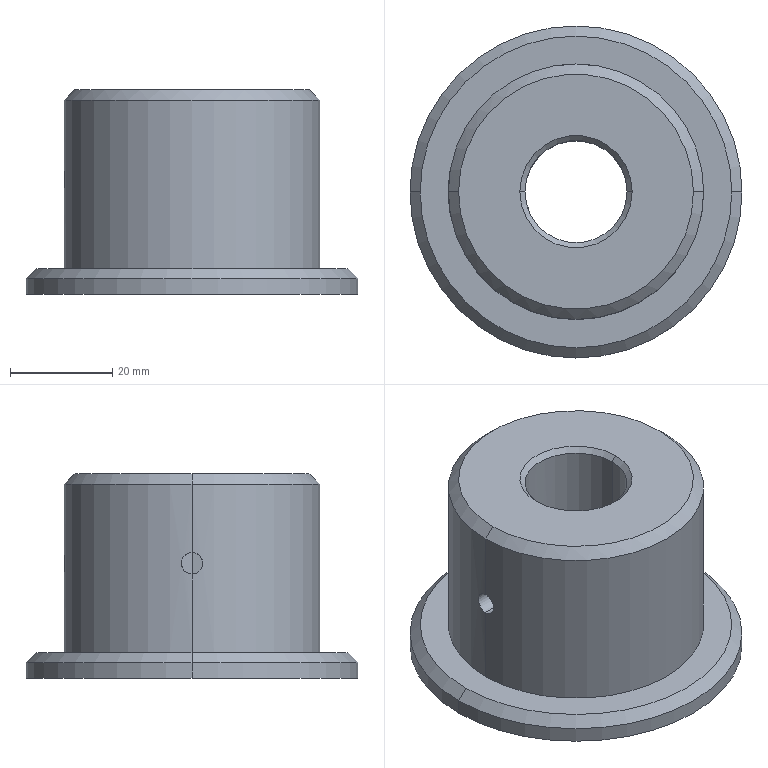Part | SolidWorks | features BaseBody 1 | 1 solid | 21 faces | box 65 x 65 x 40 mm | volume 71560 mm3 | cylinder 10 | cone 8 | plane 3 | commonest cylinder face diameters 4.2 x4 20 x2 50 x2 65 x2
STEP:
#1=CARTESIAN_POINT('',(0.,10.,24.6));
#2=VERTEX_POINT('',#1);
#3=CARTESIAN_POINT('',(0.,10.,20.4));
#4=VERTEX_POINT('',#3);
#5=CARTESIAN_POINT('',(0.,10.,24.6));
#6=CARTESIAN_POINT('',(-0.1391,10.,24.6));
#7=CARTESIAN_POINT('',(-0.2759,9.997,24.586));
#8=CARTESIAN_POINT('',(-0.5447,9.986,24.533));
#9=CARTESIAN_POINT('',(-0.6783,9.978,24.492));
#10=CARTESIAN_POINT('',(-0.9324,9.957,24.387));
#11=CARTESIAN_POINT('',(-1.053,9.945,24.322));
#12=CARTESIAN_POINT('',(-1.281,9.918,24.17));
#13=CARTESIAN_POINT('',(-1.388,9.904,24.081));
#14=CARTESIAN_POINT('',(-1.678,9.86,23.792));
#15=CARTESIAN_POINT('',(-1.834,9.831,23.558));
#16=CARTESIAN_POINT('',(-1.992,9.8,23.179));
#17=CARTESIAN_POINT('',(-2.032,9.791,23.047));
#18=CARTESIAN_POINT('',(-2.086,9.78,22.776));
#19=CARTESIAN_POINT('',(-2.1,9.777,22.639));
#20=CARTESIAN_POINT('',(-2.1,9.777,22.364));
#21=CARTESIAN_POINT('',(-2.086,9.78,22.225));
#22=CARTESIAN_POINT('',(-2.033,9.791,21.955));
#23=CARTESIAN_POINT('',(-1.993,9.8,21.824));
#24=CARTESIAN_POINT('',(-1.835,9.831,21.442));
#25=CARTESIAN_POINT('',(-1.681,9.86,21.211));
#26=CARTESIAN_POINT('',(-1.388,9.904,20.918));
#27=CARTESIAN_POINT('',(-1.283,9.918,20.832));
#28=CARTESIAN_POINT('',(-1.056,9.945,20.68));
#29=CARTESIAN_POINT('',(-0.9328,9.957,20.614));
#30=CARTESIAN_POINT('',(-0.6792,9.978,20.508));
#31=CARTESIAN_POINT('',(-0.5483,9.986,20.468));
#32=CARTESIAN_POINT('',(-0.2784,9.997,20.414));
#33=CARTESIAN_POINT('',(-0.1391,10.,20.4));
#34=CARTESIAN_POINT('',(0.,10.,20.4));
#35=B_SPLINE_CURVE_WITH_KNOTS('',3,(#5,#6,#7,#8,#9,#10,#11,#12,#13,#14,#15,#16,#17,#18,#19,#20,#21,#22,#23,#24,#25,#26,#27,#28,#29,#30,#31,#32,#33,#34),.UNSPECIFIED.,.F.,.F.,(4,2,2,2,2,2,2,2,2,2,2,2,2,2,4),(0.,0.0004114,0.0008228,0.001234,0.001646,0.002468,0.00288,0.003291,0.003702,0.004114,0.004937,0.005348,0.005759,0.006171,0.006582),.UNSPECIFIED.);
#36=EDGE_CURVE('',#2,#4,#35,.T.);
#37=ORIENTED_EDGE('',*,*,#36,.T.);
#38=CARTESIAN_POINT('',(0.,25.,20.4));
#39=VERTEX_POINT('',#38);
#40=CARTESIAN_POINT('',(0.,25.,20.4));
#41=DIRECTION('',(0.,1.,0.));
#42=VECTOR('',#41,1000.);
#43=LINE('',#40,#42);
#44=EDGE_CURVE('',#4,#39,#43,.T.);
#45=ORIENTED_EDGE('',*,*,#44,.T.);
#46=CARTESIAN_POINT('',(0.,25.,24.6));
#47=VERTEX_POINT('',#46);
#48=CARTESIAN_POINT('',(0.,25.,24.6));
#49=CARTESIAN_POINT('',(-0.1388,25.,24.6));
#50=CARTESIAN_POINT('',(-0.2752,24.999,24.586));
#51=CARTESIAN_POINT('',(-0.5437,24.994,24.533));
#52=CARTESIAN_POINT('',(-0.6771,24.991,24.493));
#53=CARTESIAN_POINT('',(-0.9313,24.983,24.387));
#54=CARTESIAN_POINT('',(-1.052,24.978,24.323));
#55=CARTESIAN_POINT('',(-1.28,24.967,24.17));
#56=CARTESIAN_POINT('',(-1.388,24.962,24.082));
#57=CARTESIAN_POINT('',(-1.679,24.944,23.791));
#58=CARTESIAN_POINT('',(-1.835,24.933,23.557));
#59=CARTESIAN_POINT('',(-2.045,24.916,23.052));
#60=CARTESIAN_POINT('',(-2.1,24.912,22.775));
#61=CARTESIAN_POINT('',(-2.1,24.912,22.364));
#62=CARTESIAN_POINT('',(-2.086,24.913,22.225));
#63=CARTESIAN_POINT('',(-2.033,24.917,21.956));
#64=CARTESIAN_POINT('',(-1.993,24.92,21.825));
#65=CARTESIAN_POINT('',(-1.888,24.929,21.571));
#66=CARTESIAN_POINT('',(-1.823,24.934,21.448));
#67=CARTESIAN_POINT('',(-1.671,24.944,21.22));
#68=CARTESIAN_POINT('',(-1.584,24.95,21.114));
#69=CARTESIAN_POINT('',(-1.388,24.962,20.918));
#70=CARTESIAN_POINT('',(-1.282,24.967,20.831));
#71=CARTESIAN_POINT('',(-1.055,24.978,20.679));
#72=CARTESIAN_POINT('',(-0.932,24.983,20.613));
#73=CARTESIAN_POINT('',(-0.6777,24.991,20.508));
#74=CARTESIAN_POINT('',(-0.5468,24.994,20.468));
#75=CARTESIAN_POINT('',(-0.2777,24.999,20.414));
#76=CARTESIAN_POINT('',(-0.1388,25.,20.4));
#77=CARTESIAN_POINT('',(0.,25.,20.4));
#78=B_SPLINE_CURVE_WITH_KNOTS('',3,(#48,#49,#50,#51,#52,#53,#54,#55,#56,#57,#58,#59,#60,#61,#62,#63,#64,#65,#66,#67,#68,#69,#70,#71,#72,#73,#74,#75,#76,#77),.UNSPECIFIED.,.F.,.F.,(4,2,2,2,2,2,2,2,2,2,2,2,2,2,4),(0.,0.0004104,0.0008209,0.001231,0.001642,0.002463,0.003284,0.003694,0.004104,0.004515,0.004925,0.005336,0.005746,0.006157,0.006567),.UNSPECIFIED.);
#79=EDGE_CURVE('',#47,#39,#78,.T.);
#80=ORIENTED_EDGE('',*,*,#79,.F.);
#81=CARTESIAN_POINT('',(0.,25.,24.6));
#82=DIRECTION('',(0.,1.,0.));
#83=VECTOR('',#82,1000.);
#84=LINE('',#81,#83);
#85=EDGE_CURVE('',#2,#47,#84,.T.);
#86=ORIENTED_EDGE('',*,*,#85,.F.);
#87=EDGE_LOOP('',(#37,#45,#80,#86));
#88=FACE_OUTER_BOUND('',#87,.T.);
#89=CARTESIAN_POINT('',(0.,25.,22.5));
#90=DIRECTION('',(0.,1.,0.));
#91=DIRECTION('',(0.,0.,1.));
#92=AXIS2_PLACEMENT_3D('',#89,#90,#91);
#93=CYLINDRICAL_SURFACE('',#92,2.1);
#94=ADVANCED_FACE('',(#88),#93,.F.);
#95=CARTESIAN_POINT('',(-10.,0.,24.6));
#96=VERTEX_POINT('',#95);
#97=CARTESIAN_POINT('',(-10.,0.,20.4));
#98=VERTEX_POINT('',#97);
#99=CARTESIAN_POINT('',(-10.,0.,24.6));
#100=CARTESIAN_POINT('',(-10.,-0.1391,24.6));
#101=CARTESIAN_POINT('',(-9.997,-0.2759,24.586));
#102=CARTESIAN_POINT('',(-9.986,-0.5447,24.533));
#103=CARTESIAN_POINT('',(-9.978,-0.6783,24.492));
#104=CARTESIAN_POINT('',(-9.957,-0.9324,24.387));
#105=CARTESIAN_POINT('',(-9.945,-1.053,24.322));
#106=CARTESIAN_POINT('',(-9.918,-1.281,24.17));
#107=CARTESIAN_POINT('',(-9.904,-1.388,24.081));
#108=CARTESIAN_POINT('',(-9.86,-1.678,23.792));
#109=CARTESIAN_POINT('',(-9.831,-1.834,23.558));
#110=CARTESIAN_POINT('',(-9.8,-1.992,23.179));
#111=CARTESIAN_POINT('',(-9.791,-2.032,23.047));
#112=CARTESIAN_POINT('',(-9.78,-2.086,22.776));
#113=CARTESIAN_POINT('',(-9.777,-2.1,22.639));
#114=CARTESIAN_POINT('',(-9.777,-2.1,22.364));
#115=CARTESIAN_POINT('',(-9.78,-2.086,22.225));
#116=CARTESIAN_POINT('',(-9.791,-2.033,21.955));
#117=CARTESIAN_POINT('',(-9.8,-1.993,21.824));
#118=CARTESIAN_POINT('',(-9.831,-1.835,21.442));
#119=CARTESIAN_POINT('',(-9.86,-1.681,21.211));
#120=CARTESIAN_POINT('',(-9.904,-1.388,20.918));
#121=CARTESIAN_POINT('',(-9.918,-1.283,20.832));
#122=CARTESIAN_POINT('',(-9.945,-1.056,20.68));
#123=CARTESIAN_POINT('',(-9.957,-0.9328,20.614));
#124=CARTESIAN_POINT('',(-9.978,-0.6792,20.508));
#125=CARTESIAN_POINT('',(-9.986,-0.5483,20.468));
#126=CARTESIAN_POINT('',(-9.997,-0.2784,20.414));
#127=CARTESIAN_POINT('',(-10.,-0.1391,20.4));
#128=CARTESIAN_POINT('',(-10.,0.,20.4));
#129=B_SPLINE_CURVE_WITH_KNOTS('',3,(#99,#100,#101,#102,#103,#104,#105,#106,#107,#108,#109,#110,#111,#112,#113,#114,#115,#116,#117,#118,#119,#120,#121,#122,#123,#124,#125,#126,#127,#128),.UNSPECIFIED.,.F.,.F.,(4,2,2,2,2,2,2,2,2,2,2,2,2,2,4),(0.,0.0004114,0.0008228,0.001234,0.001646,0.002468,0.00288,0.003291,0.003702,0.004114,0.004937,0.005348,0.005759,0.006171,0.006582),.UNSPECIFIED.);
#130=EDGE_CURVE('',#96,#98,#129,.T.);
#131=ORIENTED_EDGE('',*,*,#130,.T.);
#132=CARTESIAN_POINT('',(-25.,0.,20.4));
#133=VERTEX_POINT('',#132);
#134=CARTESIAN_POINT('',(-25.,0.,20.4));
#135=DIRECTION('',(-1.,0.,0.));
#136=VECTOR('',#135,1000.);
#137=LINE('',#134,#136);
#138=EDGE_CURVE('',#98,#133,#137,.T.);
#139=ORIENTED_EDGE('',*,*,#138,.T.);
#140=CARTESIAN_POINT('',(-25.,0.,24.6));
#141=VERTEX_POINT('',#140);
#142=CARTESIAN_POINT('',(-25.,0.,24.6));
#143=CARTESIAN_POINT('',(-25.,-0.1388,24.6));
#144=CARTESIAN_POINT('',(-24.999,-0.2752,24.586));
#145=CARTESIAN_POINT('',(-24.994,-0.5437,24.533));
#146=CARTESIAN_POINT('',(-24.991,-0.6771,24.493));
#147=CARTESIAN_POINT('',(-24.983,-0.9313,24.387));
#148=CARTESIAN_POINT('',(-24.978,-1.052,24.323));
#149=CARTESIAN_POINT('',(-24.967,-1.28,24.17));
#150=CARTESIAN_POINT('',(-24.962,-1.388,24.082));
#151=CARTESIAN_POINT('',(-24.944,-1.679,23.791));
#152=CARTESIAN_POINT('',(-24.933,-1.835,23.557));
#153=CARTESIAN_POINT('',(-24.916,-2.045,23.052));
#154=CARTESIAN_POINT('',(-24.912,-2.1,22.775));
#155=CARTESIAN_POINT('',(-24.912,-2.1,22.364));
#156=CARTESIAN_POINT('',(-24.913,-2.086,22.225));
#157=CARTESIAN_POINT('',(-24.917,-2.033,21.956));
#158=CARTESIAN_POINT('',(-24.92,-1.993,21.825));
#159=CARTESIAN_POINT('',(-24.929,-1.888,21.571));
#160=CARTESIAN_POINT('',(-24.934,-1.823,21.448));
#161=CARTESIAN_POINT('',(-24.944,-1.671,21.22));
#162=CARTESIAN_POINT('',(-24.95,-1.584,21.114));
#163=CARTESIAN_POINT('',(-24.962,-1.388,20.918));
#164=CARTESIAN_POINT('',(-24.967,-1.282,20.831));
#165=CARTESIAN_POINT('',(-24.978,-1.055,20.679));
#166=CARTESIAN_POINT('',(-24.983,-0.932,20.613));
#167=CARTESIAN_POINT('',(-24.991,-0.6777,20.508));
#168=CARTESIAN_POINT('',(-24.994,-0.5468,20.468));
#169=CARTESIAN_POINT('',(-24.999,-0.2777,20.414));
#170=CARTESIAN_POINT('',(-25.,-0.1388,20.4));
#171=CARTESIAN_POINT('',(-25.,0.,20.4));
#172=B_SPLINE_CURVE_WITH_KNOTS('',3,(#142,#143,#144,#145,#146,#147,#148,#149,#150,#151,#152,#153,#154,#155,#156,#157,#158,#159,#160,#161,#162,#163,#164,#165,#166,#167,#168,#169,#170,#171),.UNSPECIFIED.,.F.,.F.,(4,2,2,2,2,2,2,2,2,2,2,2,2,2,4),(0.,0.0004104,0.0008209,0.001231,0.001642,0.002463,0.003284,0.003694,0.004104,0.004515,0.004925,0.005336,0.005746,0.006157,0.006567),.UNSPECIFIED.);
#173=EDGE_CURVE('',#141,#133,#172,.T.);
#174=ORIENTED_EDGE('',*,*,#173,.F.);
#175=CARTESIAN_POINT('',(-25.,0.,24.6));
#176=DIRECTION('',(-1.,0.,0.));
#177=VECTOR('',#176,1000.);
#178=LINE('',#175,#177);
#179=EDGE_CURVE('',#96,#141,#178,.T.);
#180=ORIENTED_EDGE('',*,*,#179,.F.);
#181=EDGE_LOOP('',(#131,#139,#174,#180));
#182=FACE_OUTER_BOUND('',#181,.T.);
#183=CARTESIAN_POINT('',(-25.,0.,22.5));
#184=DIRECTION('',(-1.,0.,0.));
#185=DIRECTION('',(0.,0.,1.));
#186=AXIS2_PLACEMENT_3D('',#183,#184,#185);
#187=CYLINDRICAL_SURFACE('',#186,2.1);
#188=ADVANCED_FACE('',(#182),#187,.F.);
#189=CARTESIAN_POINT('',(10.,0.,1.));
#190=VERTEX_POINT('',#189);
#191=CARTESIAN_POINT('',(-10.,0.,1.));
#192=VERTEX_POINT('',#191);
#193=CARTESIAN_POINT('',(0.,0.,1.));
#194=DIRECTION('',(0.,0.,-1.));
#195=DIRECTION('',(1.,0.,0.));
#196=AXIS2_PLACEMENT_3D('',#193,#194,#195);
#197=CIRCLE('',#196,10.);
#198=EDGE_CURVE('',#190,#192,#197,.T.);
#199=ORIENTED_EDGE('',*,*,#198,.F.);
#200=CARTESIAN_POINT('',(11.,0.,0.));
#201=VERTEX_POINT('',#200);
#202=CARTESIAN_POINT('',(11.,0.,0.));
#203=DIRECTION('',(0.7071,0.,-0.7071));
#204=VECTOR('',#203,1000.);
#205=LINE('',#202,#204);
#206=EDGE_CURVE('',#190,#201,#205,.T.);
#207=ORIENTED_EDGE('',*,*,#206,.T.);
#208=CARTESIAN_POINT('',(-11.,0.,0.));
#209=VERTEX_POINT('',#208);
#210=CARTESIAN_POINT('',(0.,0.,0.));
#211=DIRECTION('',(0.,0.,1.));
#212=DIRECTION('',(1.,0.,0.));
#213=AXIS2_PLACEMENT_3D('',#210,#211,#212);
#214=CIRCLE('',#213,11.);
#215=EDGE_CURVE('',#209,#201,#214,.T.);
#216=ORIENTED_EDGE('',*,*,#215,.F.);
#217=CARTESIAN_POINT('',(-11.,0.,0.));
#218=DIRECTION('',(-0.7071,0.,-0.7071));
#219=VECTOR('',#218,1000.);
#220=LINE('',#217,#219);
#221=EDGE_CURVE('',#192,#209,#220,.T.);
#222=ORIENTED_EDGE('',*,*,#221,.F.);
#223=EDGE_LOOP('',(#199,#207,#216,#222));
#224=FACE_OUTER_BOUND('',#223,.T.);
#225=CARTESIAN_POINT('',(0.,0.,0.));
#226=DIRECTION('',(0.,0.,-1.));
#227=DIRECTION('',(-1.,0.,0.));
#228=AXIS2_PLACEMENT_3D('',#225,#226,#227);
#229=CONICAL_SURFACE('',#228,11.,0.7854);
#230=ADVANCED_FACE('',(#224),#229,.F.);
#231=CARTESIAN_POINT('',(-10.,0.,39.));
#232=VERTEX_POINT('',#231);
#233=CARTESIAN_POINT('',(10.,0.,39.));
#234=VERTEX_POINT('',#233);
#235=CARTESIAN_POINT('',(0.,0.,39.));
#236=DIRECTION('',(0.,0.,1.));
#237=DIRECTION('',(1.,0.,0.));
#238=AXIS2_PLACEMENT_3D('',#235,#236,#237);
#239=CIRCLE('',#238,10.);
#240=EDGE_CURVE('',#232,#234,#239,.T.);
#241=ORIENTED_EDGE('',*,*,#240,.F.);
#242=CARTESIAN_POINT('',(-11.,0.,40.));
#243=VERTEX_POINT('',#242);
#244=CARTESIAN_POINT('',(-10.,0.,39.));
#245=DIRECTION('',(-0.7071,0.,0.7071));
#246=VECTOR('',#245,1000.);
#247=LINE('',#244,#246);
#248=EDGE_CURVE('',#232,#243,#247,.T.);
#249=ORIENTED_EDGE('',*,*,#248,.T.);
#250=CARTESIAN_POINT('',(11.,0.,40.));
#251=VERTEX_POINT('',#250);
#252=CARTESIAN_POINT('',(0.,0.,40.));
#253=DIRECTION('',(0.,0.,-1.));
#254=DIRECTION('',(1.,0.,0.));
#255=AXIS2_PLACEMENT_3D('',#252,#253,#254);
#256=CIRCLE('',#255,11.);
#257=EDGE_CURVE('',#251,#243,#256,.T.);
#258=ORIENTED_EDGE('',*,*,#257,.F.);
#259=CARTESIAN_POINT('',(10.,0.,39.));
#260=DIRECTION('',(0.7071,0.,0.7071));
#261=VECTOR('',#260,1000.);
#262=LINE('',#259,#261);
#263=EDGE_CURVE('',#234,#251,#262,.T.);
#264=ORIENTED_EDGE('',*,*,#263,.F.);
#265=EDGE_LOOP('',(#241,#249,#258,#264));
#266=FACE_OUTER_BOUND('',#265,.T.);
#267=CARTESIAN_POINT('',(0.,0.,39.));
#268=DIRECTION('',(0.,0.,1.));
#269=DIRECTION('',(1.,0.,0.));
#270=AXIS2_PLACEMENT_3D('',#267,#268,#269);
#271=CONICAL_SURFACE('',#270,10.,0.7854);
#272=ADVANCED_FACE('',(#266),#271,.F.);
#273=CARTESIAN_POINT('',(23.,0.,40.));
#274=VERTEX_POINT('',#273);
#275=CARTESIAN_POINT('',(-23.,0.,40.));
#276=VERTEX_POINT('',#275);
#277=CARTESIAN_POINT('',(0.,0.,40.));
#278=DIRECTION('',(0.,0.,1.));
#279=DIRECTION('',(1.,0.,0.));
#280=AXIS2_PLACEMENT_3D('',#277,#278,#279);
#281=CIRCLE('',#280,23.);
#282=EDGE_CURVE('',#274,#276,#281,.T.);
#283=ORIENTED_EDGE('',*,*,#282,.F.);
#284=CARTESIAN_POINT('',(25.,0.,38.));
#285=VERTEX_POINT('',#284);
#286=CARTESIAN_POINT('',(23.,0.,40.));
#287=DIRECTION('',(0.7071,0.,-0.7071));
#288=VECTOR('',#287,1000.);
#289=LINE('',#286,#288);
#290=EDGE_CURVE('',#274,#285,#289,.T.);
#291=ORIENTED_EDGE('',*,*,#290,.T.);
#292=CARTESIAN_POINT('',(-25.,0.,38.));
#293=VERTEX_POINT('',#292);
#294=CARTESIAN_POINT('',(0.,0.,38.));
#295=DIRECTION('',(0.,0.,-1.));
#296=DIRECTION('',(1.,0.,0.));
#297=AXIS2_PLACEMENT_3D('',#294,#295,#296);
#298=CIRCLE('',#297,25.);
#299=EDGE_CURVE('',#293,#285,#298,.T.);
#300=ORIENTED_EDGE('',*,*,#299,.F.);
#301=CARTESIAN_POINT('',(-23.,0.,40.));
#302=DIRECTION('',(-0.7071,0.,-0.7071));
#303=VECTOR('',#302,1000.);
#304=LINE('',#301,#303);
#305=EDGE_CURVE('',#276,#293,#304,.T.);
#306=ORIENTED_EDGE('',*,*,#305,.F.);
#307=EDGE_LOOP('',(#283,#291,#300,#306));
#308=FACE_OUTER_BOUND('',#307,.T.);
#309=CARTESIAN_POINT('',(0.,0.,40.));
#310=DIRECTION('',(0.,0.,-1.));
#311=DIRECTION('',(-1.,0.,0.));
#312=AXIS2_PLACEMENT_3D('',#309,#310,#311);
#313=CONICAL_SURFACE('',#312,23.,0.7854);
#314=ADVANCED_FACE('',(#308),#313,.T.);
#315=CARTESIAN_POINT('',(30.5,0.,5.));
#316=VERTEX_POINT('',#315);
#317=CARTESIAN_POINT('',(-30.5,0.,5.));
#318=VERTEX_POINT('',#317);
#319=CARTESIAN_POINT('',(0.,0.,5.));
#320=DIRECTION('',(0.,0.,1.));
#321=DIRECTION('',(1.,0.,0.));
#322=AXIS2_PLACEMENT_3D('',#319,#320,#321);
#323=CIRCLE('',#322,30.5);
#324=EDGE_CURVE('',#316,#318,#323,.T.);
#325=ORIENTED_EDGE('',*,*,#324,.F.);
#326=CARTESIAN_POINT('',(32.5,0.,3.));
#327=VERTEX_POINT('',#326);
#328=CARTESIAN_POINT('',(30.5,0.,5.));
#329=DIRECTION('',(0.7071,0.,-0.7071));
#330=VECTOR('',#329,1000.);
#331=LINE('',#328,#330);
#332=EDGE_CURVE('',#316,#327,#331,.T.);
#333=ORIENTED_EDGE('',*,*,#332,.T.);
#334=CARTESIAN_POINT('',(-32.5,0.,3.));
#335=VERTEX_POINT('',#334);
#336=CARTESIAN_POINT('',(0.,0.,3.));
#337=DIRECTION('',(0.,0.,-1.));
#338=DIRECTION('',(1.,0.,0.));
#339=AXIS2_PLACEMENT_3D('',#336,#337,#338);
#340=CIRCLE('',#339,32.5);
#341=EDGE_CURVE('',#335,#327,#340,.T.);
#342=ORIENTED_EDGE('',*,*,#341,.F.);
#343=CARTESIAN_POINT('',(-30.5,0.,5.));
#344=DIRECTION('',(-0.7071,0.,-0.7071));
#345=VECTOR('',#344,1000.);
#346=LINE('',#343,#345);
#347=EDGE_CURVE('',#318,#335,#346,.T.);
#348=ORIENTED_EDGE('',*,*,#347,.F.);
#349=EDGE_LOOP('',(#325,#333,#342,#348));
#350=FACE_OUTER_BOUND('',#349,.T.);
#351=CARTESIAN_POINT('',(0.,0.,5.));
#352=DIRECTION('',(0.,0.,-1.));
#353=DIRECTION('',(-1.,0.,0.));
#354=AXIS2_PLACEMENT_3D('',#351,#352,#353);
#355=CONICAL_SURFACE('',#354,30.5,0.7854);
#356=ADVANCED_FACE('',(#350),#355,.T.);
#357=ORIENTED_EDGE('',*,*,#240,.T.);
#358=CARTESIAN_POINT('',(10.,0.,40.));
#359=DIRECTION('',(0.,0.,-1.));
#360=VECTOR('',#359,1000.);
#361=LINE('',#358,#360);
#362=EDGE_CURVE('',#234,#190,#361,.T.);
#363=ORIENTED_EDGE('',*,*,#362,.T.);
#364=ORIENTED_EDGE('',*,*,#198,.T.);
#365=CARTESIAN_POINT('',(-10.,0.,40.));
#366=DIRECTION('',(0.,0.,-1.));
#367=VECTOR('',#366,1000.);
#368=LINE('',#365,#367);
#369=EDGE_CURVE('',#98,#192,#368,.T.);
#370=ORIENTED_EDGE('',*,*,#369,.F.);
#371=ORIENTED_EDGE('',*,*,#130,.F.);
#372=CARTESIAN_POINT('',(-10.,0.,40.));
#373=DIRECTION('',(0.,0.,-1.));
#374=VECTOR('',#373,1000.);
#375=LINE('',#372,#374);
#376=EDGE_CURVE('',#232,#96,#375,.T.);
#377=ORIENTED_EDGE('',*,*,#376,.F.);
#378=EDGE_LOOP('',(#357,#363,#364,#370,#371,#377));
#379=FACE_OUTER_BOUND('',#378,.T.);
#380=CARTESIAN_POINT('',(0.,0.,40.));
#381=DIRECTION('',(0.,0.,-1.));
#382=DIRECTION('',(-1.,0.,0.));
#383=AXIS2_PLACEMENT_3D('',#380,#381,#382);
#384=CYLINDRICAL_SURFACE('',#383,10.);
#385=ADVANCED_FACE('',(#379),#384,.F.);
#386=ORIENTED_EDGE('',*,*,#79,.T.);
#387=CARTESIAN_POINT('',(0.,25.,20.4));
#388=CARTESIAN_POINT('',(0.1388,25.,20.4));
#389=CARTESIAN_POINT('',(0.2752,24.999,20.414));
#390=CARTESIAN_POINT('',(0.5437,24.994,20.467));
#391=CARTESIAN_POINT('',(0.6771,24.991,20.507));
#392=CARTESIAN_POINT('',(0.9313,24.983,20.613));
#393=CARTESIAN_POINT('',(1.052,24.978,20.677));
#394=CARTESIAN_POINT('',(1.28,24.967,20.83));
#395=CARTESIAN_POINT('',(1.388,24.962,20.918));
#396=CARTESIAN_POINT('',(1.679,24.944,21.209));
#397=CARTESIAN_POINT('',(1.835,24.933,21.443));
#398=CARTESIAN_POINT('',(2.045,24.916,21.948));
#399=CARTESIAN_POINT('',(2.1,24.912,22.225));
#400=CARTESIAN_POINT('',(2.1,24.912,22.636));
#401=CARTESIAN_POINT('',(2.086,24.913,22.775));
#402=CARTESIAN_POINT('',(2.033,24.917,23.044));
#403=CARTESIAN_POINT('',(1.993,24.92,23.175));
#404=CARTESIAN_POINT('',(1.888,24.929,23.429));
#405=CARTESIAN_POINT('',(1.823,24.934,23.552));
#406=CARTESIAN_POINT('',(1.671,24.944,23.78));
#407=CARTESIAN_POINT('',(1.584,24.95,23.886));
#408=CARTESIAN_POINT('',(1.388,24.962,24.082));
#409=CARTESIAN_POINT('',(1.282,24.967,24.169));
#410=CARTESIAN_POINT('',(1.055,24.978,24.321));
#411=CARTESIAN_POINT('',(0.932,24.983,24.387));
#412=CARTESIAN_POINT('',(0.6777,24.991,24.492));
#413=CARTESIAN_POINT('',(0.5468,24.994,24.532));
#414=CARTESIAN_POINT('',(0.2777,24.999,24.586));
#415=CARTESIAN_POINT('',(0.1388,25.,24.6));
#416=CARTESIAN_POINT('',(0.,25.,24.6));
#417=B_SPLINE_CURVE_WITH_KNOTS('',3,(#387,#388,#389,#390,#391,#392,#393,#394,#395,#396,#397,#398,#399,#400,#401,#402,#403,#404,#405,#406,#407,#408,#409,#410,#411,#412,#413,#414,#415,#416),.UNSPECIFIED.,.F.,.F.,(4,2,2,2,2,2,2,2,2,2,2,2,2,2,4),(0.006567,0.006977,0.007388,0.007798,0.008209,0.00903,0.009851,0.01026,0.01067,0.01108,0.01149,0.0119,0.01231,0.01272,0.01313),.UNSPECIFIED.);
#418=EDGE_CURVE('',#39,#47,#417,.T.);
#419=ORIENTED_EDGE('',*,*,#418,.T.);
#420=EDGE_LOOP('',(#386,#419));
#421=FACE_BOUND('',#420,.T.);
#422=ORIENTED_EDGE('',*,*,#299,.T.);
#423=CARTESIAN_POINT('',(25.,0.,5.));
#424=VERTEX_POINT('',#423);
#425=CARTESIAN_POINT('',(25.,0.,40.));
#426=DIRECTION('',(0.,0.,-1.));
#427=VECTOR('',#426,1000.);
#428=LINE('',#425,#427);
#429=EDGE_CURVE('',#285,#424,#428,.T.);
#430=ORIENTED_EDGE('',*,*,#429,.T.);
#431=CARTESIAN_POINT('',(-25.,0.,5.));
#432=VERTEX_POINT('',#431);
#433=CARTESIAN_POINT('',(0.,0.,5.));
#434=DIRECTION('',(0.,0.,1.));
#435=DIRECTION('',(1.,0.,0.));
#436=AXIS2_PLACEMENT_3D('',#433,#434,#435);
#437=CIRCLE('',#436,25.);
#438=EDGE_CURVE('',#424,#432,#437,.T.);
#439=ORIENTED_EDGE('',*,*,#438,.T.);
#440=CARTESIAN_POINT('',(-25.,0.,40.));
#441=DIRECTION('',(0.,0.,-1.));
#442=VECTOR('',#441,1000.);
#443=LINE('',#440,#442);
#444=EDGE_CURVE('',#133,#432,#443,.T.);
#445=ORIENTED_EDGE('',*,*,#444,.F.);
#446=CARTESIAN_POINT('',(-25.,0.,20.4));
#447=CARTESIAN_POINT('',(-25.,0.1388,20.4));
#448=CARTESIAN_POINT('',(-24.999,0.2752,20.414));
#449=CARTESIAN_POINT('',(-24.994,0.5437,20.467));
#450=CARTESIAN_POINT('',(-24.991,0.6771,20.507));
#451=CARTESIAN_POINT('',(-24.983,0.9313,20.613));
#452=CARTESIAN_POINT('',(-24.978,1.052,20.677));
#453=CARTESIAN_POINT('',(-24.967,1.28,20.83));
#454=CARTESIAN_POINT('',(-24.962,1.388,20.918));
#455=CARTESIAN_POINT('',(-24.944,1.679,21.209));
#456=CARTESIAN_POINT('',(-24.933,1.835,21.443));
#457=CARTESIAN_POINT('',(-24.916,2.045,21.948));
#458=CARTESIAN_POINT('',(-24.912,2.1,22.225));
#459=CARTESIAN_POINT('',(-24.912,2.1,22.636));
#460=CARTESIAN_POINT('',(-24.913,2.086,22.775));
#461=CARTESIAN_POINT('',(-24.917,2.033,23.044));
#462=CARTESIAN_POINT('',(-24.92,1.993,23.175));
#463=CARTESIAN_POINT('',(-24.929,1.888,23.429));
#464=CARTESIAN_POINT('',(-24.934,1.823,23.552));
#465=CARTESIAN_POINT('',(-24.944,1.671,23.78));
#466=CARTESIAN_POINT('',(-24.95,1.584,23.886));
#467=CARTESIAN_POINT('',(-24.962,1.388,24.082));
#468=CARTESIAN_POINT('',(-24.967,1.282,24.169));
#469=CARTESIAN_POINT('',(-24.978,1.055,24.321));
#470=CARTESIAN_POINT('',(-24.983,0.932,24.387));
#471=CARTESIAN_POINT('',(-24.991,0.6777,24.492));
#472=CARTESIAN_POINT('',(-24.994,0.5468,24.532));
#473=CARTESIAN_POINT('',(-24.999,0.2777,24.586));
#474=CARTESIAN_POINT('',(-25.,0.1388,24.6));
#475=CARTESIAN_POINT('',(-25.,0.,24.6));
#476=B_SPLINE_CURVE_WITH_KNOTS('',3,(#446,#447,#448,#449,#450,#451,#452,#453,#454,#455,#456,#457,#458,#459,#460,#461,#462,#463,#464,#465,#466,#467,#468,#469,#470,#471,#472,#473,#474,#475),.UNSPECIFIED.,.F.,.F.,(4,2,2,2,2,2,2,2,2,2,2,2,2,2,4),(0.006567,0.006977,0.007388,0.007798,0.008209,0.00903,0.009851,0.01026,0.01067,0.01108,0.01149,0.0119,0.01231,0.01272,0.01313),.UNSPECIFIED.);
#477=EDGE_CURVE('',#133,#141,#476,.T.);
#478=ORIENTED_EDGE('',*,*,#477,.T.);
#479=CARTESIAN_POINT('',(-25.,0.,40.));
#480=DIRECTION('',(0.,0.,-1.));
#481=VECTOR('',#480,1000.);
#482=LINE('',#479,#481);
#483=EDGE_CURVE('',#293,#141,#482,.T.);
#484=ORIENTED_EDGE('',*,*,#483,.F.);
#485=EDGE_LOOP('',(#422,#430,#439,#445,#478,#484));
#486=FACE_OUTER_BOUND('',#485,.T.);
#487=CARTESIAN_POINT('',(0.,0.,40.));
#488=DIRECTION('',(0.,0.,-1.));
#489=DIRECTION('',(-1.,0.,0.));
#490=AXIS2_PLACEMENT_3D('',#487,#488,#489);
#491=CYLINDRICAL_SURFACE('',#490,25.);
#492=ADVANCED_FACE('',(#421,#486),#491,.T.);
#493=ORIENTED_EDGE('',*,*,#341,.T.);
#494=CARTESIAN_POINT('',(32.5,0.,0.));
#495=VERTEX_POINT('',#494);
#496=CARTESIAN_POINT('',(32.5,0.,5.));
#497=DIRECTION('',(0.,0.,-1.));
#498=VECTOR('',#497,1000.);
#499=LINE('',#496,#498);
#500=EDGE_CURVE('',#327,#495,#499,.T.);
#501=ORIENTED_EDGE('',*,*,#500,.T.);
#502=CARTESIAN_POINT('',(-32.5,0.,0.));
#503=VERTEX_POINT('',#502);
#504=CARTESIAN_POINT('',(0.,0.,0.));
#505=DIRECTION('',(0.,0.,1.));
#506=DIRECTION('',(1.,0.,0.));
#507=AXIS2_PLACEMENT_3D('',#504,#505,#506);
#508=CIRCLE('',#507,32.5);
#509=EDGE_CURVE('',#495,#503,#508,.T.);
#510=ORIENTED_EDGE('',*,*,#509,.T.);
#511=CARTESIAN_POINT('',(-32.5,0.,5.));
#512=DIRECTION('',(0.,0.,-1.));
#513=VECTOR('',#512,1000.);
#514=LINE('',#511,#513);
#515=EDGE_CURVE('',#335,#503,#514,.T.);
#516=ORIENTED_EDGE('',*,*,#515,.F.);
#517=EDGE_LOOP('',(#493,#501,#510,#516));
#518=FACE_OUTER_BOUND('',#517,.T.);
#519=CARTESIAN_POINT('',(0.,0.,5.));
#520=DIRECTION('',(0.,0.,-1.));
#521=DIRECTION('',(-1.,0.,0.));
#522=AXIS2_PLACEMENT_3D('',#519,#520,#521);
#523=CYLINDRICAL_SURFACE('',#522,32.5);
#524=ADVANCED_FACE('',(#518),#523,.T.);
#525=ORIENTED_EDGE('',*,*,#257,.T.);
#526=CARTESIAN_POINT('',(0.,0.,40.));
#527=DIRECTION('',(0.,0.,-1.));
#528=DIRECTION('',(1.,0.,0.));
#529=AXIS2_PLACEMENT_3D('',#526,#527,#528);
#530=CIRCLE('',#529,11.);
#531=EDGE_CURVE('',#243,#251,#530,.T.);
#532=ORIENTED_EDGE('',*,*,#531,.T.);
#533=EDGE_LOOP('',(#525,#532));
#534=FACE_BOUND('',#533,.T.);
#535=CARTESIAN_POINT('',(0.,0.,40.));
#536=DIRECTION('',(0.,0.,1.));
#537=DIRECTION('',(1.,0.,0.));
#538=AXIS2_PLACEMENT_3D('',#535,#536,#537);
#539=CIRCLE('',#538,23.);
#540=EDGE_CURVE('',#276,#274,#539,.T.);
#541=ORIENTED_EDGE('',*,*,#540,.T.);
#542=ORIENTED_EDGE('',*,*,#282,.T.);
#543=EDGE_LOOP('',(#541,#542));
#544=FACE_OUTER_BOUND('',#543,.T.);
#545=CARTESIAN_POINT('',(0.,0.,40.));
#546=DIRECTION('',(0.,0.,1.));
#547=DIRECTION('',(1.,0.,0.));
#548=AXIS2_PLACEMENT_3D('',#545,#546,#547);
#549=PLANE('',#548);
#550=ADVANCED_FACE('',(#534,#544),#549,.T.);
#551=ORIENTED_EDGE('',*,*,#215,.T.);
#552=CARTESIAN_POINT('',(0.,0.,0.));
#553=DIRECTION('',(0.,0.,1.));
#554=DIRECTION('',(1.,0.,0.));
#555=AXIS2_PLACEMENT_3D('',#552,#553,#554);
#556=CIRCLE('',#555,11.);
#557=EDGE_CURVE('',#201,#209,#556,.T.);
#558=ORIENTED_EDGE('',*,*,#557,.T.);
#559=EDGE_LOOP('',(#551,#558));
#560=FACE_BOUND('',#559,.T.);
#561=CARTESIAN_POINT('',(0.,0.,0.));
#562=DIRECTION('',(0.,0.,1.));
#563=DIRECTION('',(1.,0.,0.));
#564=AXIS2_PLACEMENT_3D('',#561,#562,#563);
#565=CIRCLE('',#564,32.5);
#566=EDGE_CURVE('',#503,#495,#565,.T.);
#567=ORIENTED_EDGE('',*,*,#566,.F.);
#568=ORIENTED_EDGE('',*,*,#509,.F.);
#569=EDGE_LOOP('',(#567,#568));
#570=FACE_OUTER_BOUND('',#569,.T.);
#571=CARTESIAN_POINT('',(0.,0.,0.));
#572=DIRECTION('',(0.,0.,1.));
#573=DIRECTION('',(1.,0.,0.));
#574=AXIS2_PLACEMENT_3D('',#571,#572,#573);
#575=PLANE('',#574);
#576=ADVANCED_FACE('',(#560,#570),#575,.F.);
#577=CARTESIAN_POINT('',(0.,0.,5.));
#578=DIRECTION('',(0.,0.,1.));
#579=DIRECTION('',(1.,0.,0.));
#580=AXIS2_PLACEMENT_3D('',#577,#578,#579);
#581=CIRCLE('',#580,25.);
#582=EDGE_CURVE('',#432,#424,#581,.T.);
#583=ORIENTED_EDGE('',*,*,#582,.F.);
#584=ORIENTED_EDGE('',*,*,#438,.F.);
#585=EDGE_LOOP('',(#583,#584));
#586=FACE_BOUND('',#585,.T.);
#587=CARTESIAN_POINT('',(0.,0.,5.));
#588=DIRECTION('',(0.,0.,1.));
#589=DIRECTION('',(1.,0.,0.));
#590=AXIS2_PLACEMENT_3D('',#587,#588,#589);
#591=CIRCLE('',#590,30.5);
#592=EDGE_CURVE('',#318,#316,#591,.T.);
#593=ORIENTED_EDGE('',*,*,#592,.T.);
#594=ORIENTED_EDGE('',*,*,#324,.T.);
#595=EDGE_LOOP('',(#593,#594));
#596=FACE_OUTER_BOUND('',#595,.T.);
#597=CARTESIAN_POINT('',(0.,0.,5.));
#598=DIRECTION('',(0.,0.,1.));
#599=DIRECTION('',(1.,0.,0.));
#600=AXIS2_PLACEMENT_3D('',#597,#598,#599);
#601=PLANE('',#600);
#602=ADVANCED_FACE('',(#586,#596),#601,.T.);
#603=ORIENTED_EDGE('',*,*,#500,.F.);
#604=CARTESIAN_POINT('',(0.,0.,3.));
#605=DIRECTION('',(0.,0.,-1.));
#606=DIRECTION('',(1.,0.,0.));
#607=AXIS2_PLACEMENT_3D('',#604,#605,#606);
#608=CIRCLE('',#607,32.5);
#609=EDGE_CURVE('',#327,#335,#608,.T.);
#610=ORIENTED_EDGE('',*,*,#609,.T.);
#611=ORIENTED_EDGE('',*,*,#515,.T.);
#612=ORIENTED_EDGE('',*,*,#566,.T.);
#613=EDGE_LOOP('',(#603,#610,#611,#612));
#614=FACE_OUTER_BOUND('',#613,.T.);
#615=CARTESIAN_POINT('',(0.,0.,5.));
#616=DIRECTION('',(0.,0.,-1.));
#617=DIRECTION('',(-1.,0.,0.));
#618=AXIS2_PLACEMENT_3D('',#615,#616,#617);
#619=CYLINDRICAL_SURFACE('',#618,32.5);
#620=ADVANCED_FACE('',(#614),#619,.T.);
#621=ORIENTED_EDGE('',*,*,#429,.F.);
#622=CARTESIAN_POINT('',(0.,0.,38.));
#623=DIRECTION('',(0.,0.,-1.));
#624=DIRECTION('',(1.,0.,0.));
#625=AXIS2_PLACEMENT_3D('',#622,#623,#624);
#626=CIRCLE('',#625,25.);
#627=EDGE_CURVE('',#285,#293,#626,.T.);
#628=ORIENTED_EDGE('',*,*,#627,.T.);
#629=ORIENTED_EDGE('',*,*,#483,.T.);
#630=ORIENTED_EDGE('',*,*,#173,.T.);
#631=ORIENTED_EDGE('',*,*,#444,.T.);
#632=ORIENTED_EDGE('',*,*,#582,.T.);
#633=EDGE_LOOP('',(#621,#628,#629,#630,#631,#632));
#634=FACE_OUTER_BOUND('',#633,.T.);
#635=CARTESIAN_POINT('',(0.,0.,40.));
#636=DIRECTION('',(0.,0.,-1.));
#637=DIRECTION('',(-1.,0.,0.));
#638=AXIS2_PLACEMENT_3D('',#635,#636,#637);
#639=CYLINDRICAL_SURFACE('',#638,25.);
#640=ADVANCED_FACE('',(#634),#639,.T.);
#641=ORIENTED_EDGE('',*,*,#362,.F.);
#642=CARTESIAN_POINT('',(0.,0.,39.));
#643=DIRECTION('',(0.,0.,1.));
#644=DIRECTION('',(1.,0.,0.));
#645=AXIS2_PLACEMENT_3D('',#642,#643,#644);
#646=CIRCLE('',#645,10.);
#647=EDGE_CURVE('',#234,#232,#646,.T.);
#648=ORIENTED_EDGE('',*,*,#647,.T.);
#649=ORIENTED_EDGE('',*,*,#376,.T.);
#650=CARTESIAN_POINT('',(-10.,0.,20.4));
#651=CARTESIAN_POINT('',(-10.,0.1391,20.4));
#652=CARTESIAN_POINT('',(-9.997,0.2759,20.414));
#653=CARTESIAN_POINT('',(-9.986,0.5447,20.467));
#654=CARTESIAN_POINT('',(-9.978,0.6783,20.508));
#655=CARTESIAN_POINT('',(-9.957,0.9324,20.613));
#656=CARTESIAN_POINT('',(-9.945,1.053,20.678));
#657=CARTESIAN_POINT('',(-9.918,1.281,20.83));
#658=CARTESIAN_POINT('',(-9.904,1.388,20.919));
#659=CARTESIAN_POINT('',(-9.86,1.678,21.208));
#660=CARTESIAN_POINT('',(-9.831,1.834,21.442));
#661=CARTESIAN_POINT('',(-9.8,1.992,21.821));
#662=CARTESIAN_POINT('',(-9.791,2.032,21.953));
#663=CARTESIAN_POINT('',(-9.78,2.086,22.224));
#664=CARTESIAN_POINT('',(-9.777,2.1,22.361));
#665=CARTESIAN_POINT('',(-9.777,2.1,22.636));
#666=CARTESIAN_POINT('',(-9.78,2.086,22.775));
#667=CARTESIAN_POINT('',(-9.791,2.033,23.045));
#668=CARTESIAN_POINT('',(-9.8,1.993,23.176));
#669=CARTESIAN_POINT('',(-9.831,1.835,23.558));
#670=CARTESIAN_POINT('',(-9.86,1.681,23.789));
#671=CARTESIAN_POINT('',(-9.904,1.388,24.082));
#672=CARTESIAN_POINT('',(-9.918,1.283,24.168));
#673=CARTESIAN_POINT('',(-9.945,1.056,24.32));
#674=CARTESIAN_POINT('',(-9.957,0.9328,24.386));
#675=CARTESIAN_POINT('',(-9.978,0.6792,24.492));
#676=CARTESIAN_POINT('',(-9.986,0.5483,24.532));
#677=CARTESIAN_POINT('',(-9.997,0.2784,24.586));
#678=CARTESIAN_POINT('',(-10.,0.1391,24.6));
#679=CARTESIAN_POINT('',(-10.,0.,24.6));
#680=B_SPLINE_CURVE_WITH_KNOTS('',3,(#650,#651,#652,#653,#654,#655,#656,#657,#658,#659,#660,#661,#662,#663,#664,#665,#666,#667,#668,#669,#670,#671,#672,#673,#674,#675,#676,#677,#678,#679),.UNSPECIFIED.,.F.,.F.,(4,2,2,2,2,2,2,2,2,2,2,2,2,2,4),(0.006582,0.006993,0.007405,0.007816,0.008228,0.00905,0.009462,0.009873,0.01028,0.0107,0.01152,0.01193,0.01234,0.01275,0.01316),.UNSPECIFIED.);
#681=EDGE_CURVE('',#98,#96,#680,.T.);
#682=ORIENTED_EDGE('',*,*,#681,.F.);
#683=ORIENTED_EDGE('',*,*,#369,.T.);
#684=CARTESIAN_POINT('',(0.,0.,1.));
#685=DIRECTION('',(0.,0.,-1.));
#686=DIRECTION('',(1.,0.,0.));
#687=AXIS2_PLACEMENT_3D('',#684,#685,#686);
#688=CIRCLE('',#687,10.);
#689=EDGE_CURVE('',#192,#190,#688,.T.);
#690=ORIENTED_EDGE('',*,*,#689,.T.);
#691=EDGE_LOOP('',(#641,#648,#649,#682,#683,#690));
#692=FACE_OUTER_BOUND('',#691,.T.);
#693=ORIENTED_EDGE('',*,*,#36,.F.);
#694=CARTESIAN_POINT('',(0.,10.,20.4));
#695=CARTESIAN_POINT('',(0.1391,10.,20.4));
#696=CARTESIAN_POINT('',(0.2759,9.997,20.414));
#697=CARTESIAN_POINT('',(0.5447,9.986,20.467));
#698=CARTESIAN_POINT('',(0.6783,9.978,20.508));
#699=CARTESIAN_POINT('',(0.9324,9.957,20.613));
#700=CARTESIAN_POINT('',(1.053,9.945,20.678));
#701=CARTESIAN_POINT('',(1.281,9.918,20.83));
#702=CARTESIAN_POINT('',(1.388,9.904,20.919));
#703=CARTESIAN_POINT('',(1.678,9.86,21.208));
#704=CARTESIAN_POINT('',(1.834,9.831,21.442));
#705=CARTESIAN_POINT('',(1.992,9.8,21.821));
#706=CARTESIAN_POINT('',(2.032,9.791,21.953));
#707=CARTESIAN_POINT('',(2.086,9.78,22.224));
#708=CARTESIAN_POINT('',(2.1,9.777,22.361));
#709=CARTESIAN_POINT('',(2.1,9.777,22.636));
#710=CARTESIAN_POINT('',(2.086,9.78,22.775));
#711=CARTESIAN_POINT('',(2.033,9.791,23.045));
#712=CARTESIAN_POINT('',(1.993,9.8,23.176));
#713=CARTESIAN_POINT('',(1.835,9.831,23.558));
#714=CARTESIAN_POINT('',(1.681,9.86,23.789));
#715=CARTESIAN_POINT('',(1.388,9.904,24.082));
#716=CARTESIAN_POINT('',(1.283,9.918,24.168));
#717=CARTESIAN_POINT('',(1.056,9.945,24.32));
#718=CARTESIAN_POINT('',(0.9328,9.957,24.386));
#719=CARTESIAN_POINT('',(0.6792,9.978,24.492));
#720=CARTESIAN_POINT('',(0.5483,9.986,24.532));
#721=CARTESIAN_POINT('',(0.2784,9.997,24.586));
#722=CARTESIAN_POINT('',(0.1391,10.,24.6));
#723=CARTESIAN_POINT('',(0.,10.,24.6));
#724=B_SPLINE_CURVE_WITH_KNOTS('',3,(#694,#695,#696,#697,#698,#699,#700,#701,#702,#703,#704,#705,#706,#707,#708,#709,#710,#711,#712,#713,#714,#715,#716,#717,#718,#719,#720,#721,#722,#723),.UNSPECIFIED.,.F.,.F.,(4,2,2,2,2,2,2,2,2,2,2,2,2,2,4),(0.006582,0.006993,0.007405,0.007816,0.008228,0.00905,0.009462,0.009873,0.01028,0.0107,0.01152,0.01193,0.01234,0.01275,0.01316),.UNSPECIFIED.);
#725=EDGE_CURVE('',#4,#2,#724,.T.);
#726=ORIENTED_EDGE('',*,*,#725,.F.);
#727=EDGE_LOOP('',(#693,#726));
#728=FACE_BOUND('',#727,.T.);
#729=CARTESIAN_POINT('',(0.,0.,40.));
#730=DIRECTION('',(0.,0.,-1.));
#731=DIRECTION('',(-1.,0.,0.));
#732=AXIS2_PLACEMENT_3D('',#729,#730,#731);
#733=CYLINDRICAL_SURFACE('',#732,10.);
#734=ADVANCED_FACE('',(#692,#728),#733,.F.);
#735=ORIENTED_EDGE('',*,*,#332,.F.);
#736=ORIENTED_EDGE('',*,*,#592,.F.);
#737=ORIENTED_EDGE('',*,*,#347,.T.);
#738=ORIENTED_EDGE('',*,*,#609,.F.);
#739=EDGE_LOOP('',(#735,#736,#737,#738));
#740=FACE_OUTER_BOUND('',#739,.T.);
#741=CARTESIAN_POINT('',(0.,0.,5.));
#742=DIRECTION('',(0.,0.,-1.));
#743=DIRECTION('',(-1.,0.,0.));
#744=AXIS2_PLACEMENT_3D('',#741,#742,#743);
#745=CONICAL_SURFACE('',#744,30.5,0.7854);
#746=ADVANCED_FACE('',(#740),#745,.T.);
#747=ORIENTED_EDGE('',*,*,#290,.F.);
#748=ORIENTED_EDGE('',*,*,#540,.F.);
#749=ORIENTED_EDGE('',*,*,#305,.T.);
#750=ORIENTED_EDGE('',*,*,#627,.F.);
#751=EDGE_LOOP('',(#747,#748,#749,#750));
#752=FACE_OUTER_BOUND('',#751,.T.);
#753=CARTESIAN_POINT('',(0.,0.,40.));
#754=DIRECTION('',(0.,0.,-1.));
#755=DIRECTION('',(-1.,0.,0.));
#756=AXIS2_PLACEMENT_3D('',#753,#754,#755);
#757=CONICAL_SURFACE('',#756,23.,0.7854);
#758=ADVANCED_FACE('',(#752),#757,.T.);
#759=ORIENTED_EDGE('',*,*,#248,.F.);
#760=ORIENTED_EDGE('',*,*,#647,.F.);
#761=ORIENTED_EDGE('',*,*,#263,.T.);
#762=ORIENTED_EDGE('',*,*,#531,.F.);
#763=EDGE_LOOP('',(#759,#760,#761,#762));
#764=FACE_OUTER_BOUND('',#763,.T.);
#765=CARTESIAN_POINT('',(0.,0.,39.));
#766=DIRECTION('',(0.,0.,1.));
#767=DIRECTION('',(1.,0.,0.));
#768=AXIS2_PLACEMENT_3D('',#765,#766,#767);
#769=CONICAL_SURFACE('',#768,10.,0.7854);
#770=ADVANCED_FACE('',(#764),#769,.F.);
#771=ORIENTED_EDGE('',*,*,#206,.F.);
#772=ORIENTED_EDGE('',*,*,#689,.F.);
#773=ORIENTED_EDGE('',*,*,#221,.T.);
#774=ORIENTED_EDGE('',*,*,#557,.F.);
#775=EDGE_LOOP('',(#771,#772,#773,#774));
#776=FACE_OUTER_BOUND('',#775,.T.);
#777=CARTESIAN_POINT('',(0.,0.,0.));
#778=DIRECTION('',(0.,0.,-1.));
#779=DIRECTION('',(-1.,0.,0.));
#780=AXIS2_PLACEMENT_3D('',#777,#778,#779);
#781=CONICAL_SURFACE('',#780,11.,0.7854);
#782=ADVANCED_FACE('',(#776),#781,.F.);
#783=ORIENTED_EDGE('',*,*,#138,.F.);
#784=ORIENTED_EDGE('',*,*,#681,.T.);
#785=ORIENTED_EDGE('',*,*,#179,.T.);
#786=ORIENTED_EDGE('',*,*,#477,.F.);
#787=EDGE_LOOP('',(#783,#784,#785,#786));
#788=FACE_OUTER_BOUND('',#787,.T.);
#789=CARTESIAN_POINT('',(-25.,0.,22.5));
#790=DIRECTION('',(-1.,0.,0.));
#791=DIRECTION('',(0.,0.,1.));
#792=AXIS2_PLACEMENT_3D('',#789,#790,#791);
#793=CYLINDRICAL_SURFACE('',#792,2.1);
#794=ADVANCED_FACE('',(#788),#793,.F.);
#795=ORIENTED_EDGE('',*,*,#44,.F.);
#796=ORIENTED_EDGE('',*,*,#725,.T.);
#797=ORIENTED_EDGE('',*,*,#85,.T.);
#798=ORIENTED_EDGE('',*,*,#418,.F.);
#799=EDGE_LOOP('',(#795,#796,#797,#798));
#800=FACE_OUTER_BOUND('',#799,.T.);
#801=CARTESIAN_POINT('',(0.,25.,22.5));
#802=DIRECTION('',(0.,1.,0.));
#803=DIRECTION('',(0.,0.,1.));
#804=AXIS2_PLACEMENT_3D('',#801,#802,#803);
#805=CYLINDRICAL_SURFACE('',#804,2.1);
#806=ADVANCED_FACE('',(#800),#805,.F.);
#807=CLOSED_SHELL('',(#94,#188,#230,#272,#314,#356,#385,#492,#524,#550,#576,#602,#620,#640,#734,#746,#758,#770,#782,#794,#806));
#808=MANIFOLD_SOLID_BREP('',#807);
#809=CARTESIAN_POINT('',(0.,0.,0.));
#810=DIRECTION('',(0.,0.,1.));
#811=DIRECTION('',(1.,0.,0.));
#812=AXIS2_PLACEMENT_3D('',#809,#810,#811);
#813=(LENGTH_UNIT()NAMED_UNIT(*)SI_UNIT(.MILLI.,.METRE.));
#814=UNCERTAINTY_MEASURE_WITH_UNIT(LENGTH_MEASURE(0.00001),#813,'','');
#815=(NAMED_UNIT(*)PLANE_ANGLE_UNIT()SI_UNIT($,.RADIAN.));
#816=(NAMED_UNIT(*)SI_UNIT($,.STERADIAN.)SOLID_ANGLE_UNIT());
#817=(GEOMETRIC_REPRESENTATION_CONTEXT(3)GLOBAL_UNCERTAINTY_ASSIGNED_CONTEXT((#814))GLOBAL_UNIT_ASSIGNED_CONTEXT((#813,#815,#816))REPRESENTATION_CONTEXT('',''));
#818=ADVANCED_BREP_SHAPE_REPRESENTATION('',(#808,#812),#817);